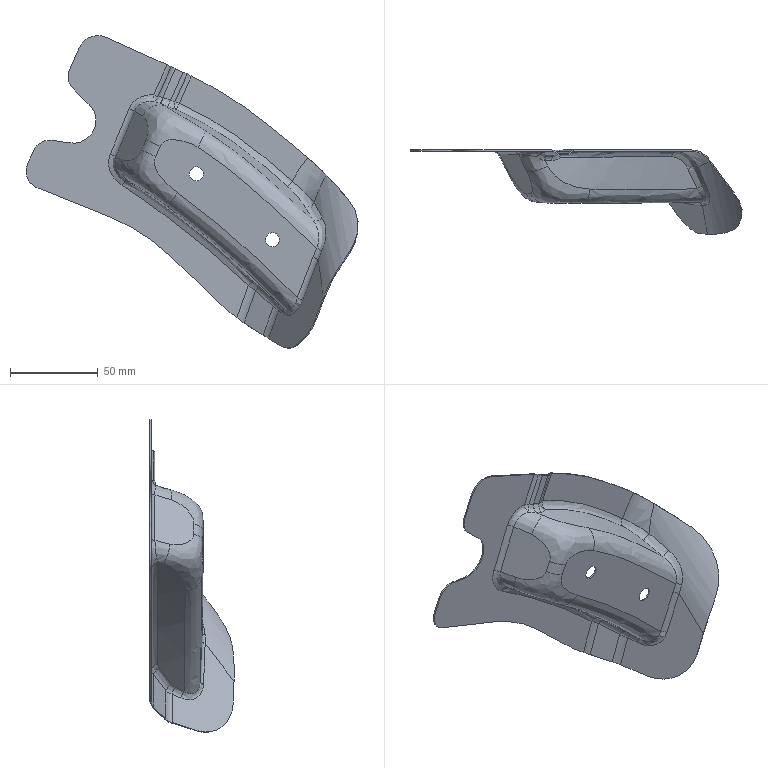Part | STEP file | FNA5401851 | 1 solid | 129 faces | box 189.152 x 47.956 x 178.015 mm | volume 18533 mm3 | spline 65 | cylinder 32 | plane 23 | other 5 | sphere 4 | commonest cylinder face diameters 8 x10 20 x6 9.6 x4 6.4 x2 21.6 x2 18.4 x1